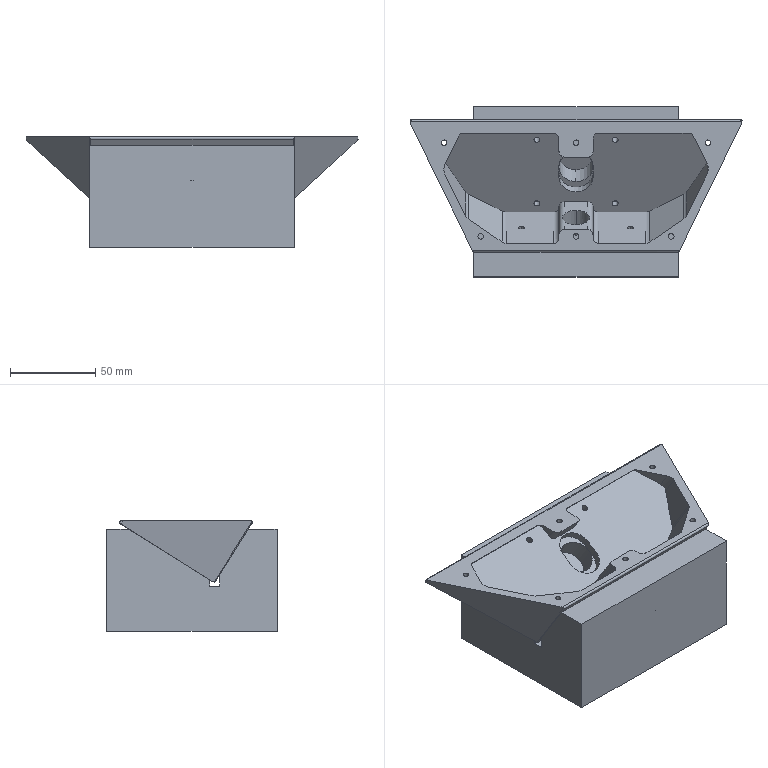NC program | Mastercam | posted with a generic post | part box 195.124 x 100 x 65 mm
Lines 1 to 1042 of 16336:
%
O0000()
(MATERIAL - ALUMINUM MM - 2024)
( T8 | 16 RC | H8 | D8 | WEAR COMP | TOOL DIA. - 16. | XY STOCK TO LEAVE - .15 | Z STOCK TO LEAVE - 0. )
( T2 | 16 FI | H2 | D2 | WEAR COMP | TOOL DIA. - 16. )
( T9 | 6 FEM | H9 | D9 | WEAR COMP | TOOL DIA. - 6. )
( T10 | 8 BM | H10 )
( T3 | 6 SPD | H3 )
( T11 | 10.3 DR | H11 )
( T12 | M12 X 1.75 RH | H12 )
( T13 | 10 FEMF | H13 | D13 | WEAR COMP | TOOL DIA. - 10. | XY STOCK TO LEAVE - .1 | Z STOCK TO LEAVE - 0. )
( T14 | 4.5 DR | H14 )
( T15 | 8 FEMR | H15 )
( T16 | 9 DR | H16 )
( T17 | 8 FEMF | H17 | D17 | WEAR COMP | TOOL DIA. - 8. | XY STOCK TO LEAVE - .05 | Z STOCK TO LEAVE - 0. )
( T18 | 14 FEM | H18 )
( T6 | 12 FEMR | H6 | XY STOCK TO LEAVE - .5 | Z STOCK TO LEAVE - .1 )
( T7 | 12 FEMF | H7 | XY STOCK TO LEAVE - .3 | Z STOCK TO LEAVE - 0. )
N100 G21
N110 G0 G17 G40 G49 G80 G90
N120 T8 M6
N130 G0 G90 G54 X82.95 Y-9.86 A0. S5500 M3
N140 G43 H8 Z50.
N150 Z1.
N160 G1 Z0. F2000.
N170 G41 D8 X68.95
N180 G3 X68.15 Y-10.66 I0. J-.8
N190 G1 Y-57.173 Z-.189
N200 G2 X60. Y-65.323 Z-.242 I-8.15 J0.
N210 G1 X-60. Z-.73
N220 G2 X-68.15 Y-57.173 Z-.782 I0. J8.15
N230 G1 Y42.828 Z-1.189
N240 G2 X-60. Y50.978 Z-1.242 I8.15 J0.
N250 G1 X60. Z-1.73
N260 G2 X68.15 Y42.828 Z-1.782 I0. J-8.15
N270 G1 Y-10.66 Z-2.
N280 Y-57.173 Z-2.189
N290 G2 X60. Y-65.323 Z-2.242 I-8.15 J0.
N300 G1 X-60. Z-2.73
N310 G2 X-68.15 Y-57.173 Z-2.782 I0. J8.15
N320 G1 Y42.828 Z-3.189
N330 G2 X-60. Y50.978 Z-3.242 I8.15 J0.
N340 G1 X60. Z-3.73
N350 G2 X68.15 Y42.828 Z-3.782 I0. J-8.15
N360 G1 Y-10.66 Z-4.
N370 Y-57.173 Z-4.189
N380 G2 X60. Y-65.323 Z-4.242 I-8.15 J0.
N390 G1 X-60. Z-4.73
N400 G2 X-68.15 Y-57.173 Z-4.782 I0. J8.15
N410 G1 Y42.828 Z-5.189
N420 G2 X-60. Y50.978 Z-5.242 I8.15 J0.
N430 G1 X60. Z-5.73
N440 G2 X68.15 Y42.828 Z-5.782 I0. J-8.15
N450 G1 Y-10.66 Z-6.
N460 Y-57.173 Z-6.189
N470 G2 X60. Y-65.323 Z-6.242 I-8.15 J0.
N480 G1 X-60. Z-6.73
N490 G2 X-68.15 Y-57.173 Z-6.782 I0. J8.15
N500 G1 Y42.828 Z-7.189
N510 G2 X-60. Y50.978 Z-7.242 I8.15 J0.
N520 G1 X60. Z-7.73
N530 G2 X68.15 Y42.828 Z-7.782 I0. J-8.15
N540 G1 Y-10.66 Z-8.
N550 Y-57.173 Z-8.189
N560 G2 X60. Y-65.323 Z-8.242 I-8.15 J0.
N570 G1 X-60. Z-8.73
N580 G2 X-68.15 Y-57.173 Z-8.782 I0. J8.15
N590 G1 Y42.828 Z-9.189
N600 G2 X-60. Y50.978 Z-9.242 I8.15 J0.
N610 G1 X60. Z-9.73
N620 G2 X68.15 Y42.828 Z-9.782 I0. J-8.15
N630 G1 Y-10.66 Z-10.
N640 Y-57.173 Z-10.189
N650 G2 X60. Y-65.323 Z-10.242 I-8.15 J0.
N660 G1 X-60. Z-10.73
N670 G2 X-68.15 Y-57.173 Z-10.782 I0. J8.15
N680 G1 Y42.828 Z-11.189
N690 G2 X-60. Y50.978 Z-11.242 I8.15 J0.
N700 G1 X60. Z-11.73
N710 G2 X68.15 Y42.828 Z-11.782 I0. J-8.15
N720 G1 Y-10.66 Z-12.
N730 Y-57.173 Z-12.189
N740 G2 X60. Y-65.323 Z-12.242 I-8.15 J0.
N750 G1 X-60. Z-12.73
N760 G2 X-68.15 Y-57.173 Z-12.782 I0. J8.15
N770 G1 Y42.828 Z-13.189
N780 G2 X-60. Y50.978 Z-13.242 I8.15 J0.
N790 G1 X60. Z-13.73
N800 G2 X68.15 Y42.828 Z-13.782 I0. J-8.15
N810 G1 Y-10.66 Z-14.
N820 Y-57.173 Z-14.189
N830 G2 X60. Y-65.323 Z-14.242 I-8.15 J0.
N840 G1 X-60. Z-14.73
N850 G2 X-68.15 Y-57.173 Z-14.782 I0. J8.15
N860 G1 Y42.828 Z-15.189
N870 G2 X-60. Y50.978 Z-15.242 I8.15 J0.
N880 G1 X60. Z-15.73
N890 G2 X68.15 Y42.828 Z-15.782 I0. J-8.15
N900 G1 Y-10.66 Z-16.
N910 Y-57.173 Z-16.189
N920 G2 X60. Y-65.323 Z-16.242 I-8.15 J0.
N930 G1 X-60. Z-16.73
N940 G2 X-68.15 Y-57.173 Z-16.782 I0. J8.15
N950 G1 Y42.828 Z-17.189
N960 G2 X-60. Y50.978 Z-17.242 I8.15 J0.
N970 G1 X60. Z-17.73
N980 G2 X68.15 Y42.828 Z-17.782 I0. J-8.15
N990 G1 Y-10.66 Z-18.
N1000 Y-57.173 Z-18.189
N1010 G2 X60. Y-65.323 Z-18.242 I-8.15 J0.
N1020 G1 X-60. Z-18.73
N1030 G2 X-68.15 Y-57.173 Z-18.782 I0. J8.15
N1040 G1 Y42.828 Z-19.189
N1050 G2 X-60. Y50.978 Z-19.242 I8.15 J0.
N1060 G1 X60. Z-19.73
N1070 G2 X68.15 Y42.828 Z-19.782 I0. J-8.15
N1080 G1 Y-10.66 Z-20.
N1090 Y-57.173 Z-20.189
N1100 G2 X60. Y-65.323 Z-20.242 I-8.15 J0.
N1110 G1 X-60. Z-20.73
N1120 G2 X-68.15 Y-57.173 Z-20.782 I0. J8.15
N1130 G1 Y42.828 Z-21.189
N1140 G2 X-60. Y50.978 Z-21.242 I8.15 J0.
N1150 G1 X60. Z-21.73
N1160 G2 X68.15 Y42.828 Z-21.782 I0. J-8.15
N1170 G1 Y-10.66 Z-22.
N1180 Y-57.173 Z-22.189
N1190 G2 X60. Y-65.323 Z-22.242 I-8.15 J0.
N1200 G1 X-60. Z-22.73
N1210 G2 X-68.15 Y-57.173 Z-22.782 I0. J8.15
N1220 G1 Y42.828 Z-23.189
N1230 G2 X-60. Y50.978 Z-23.242 I8.15 J0.
N1240 G1 X60. Z-23.73
N1250 G2 X68.15 Y42.828 Z-23.782 I0. J-8.15
N1260 G1 Y-10.66 Z-24.
N1270 Y-57.173 Z-24.189
N1280 G2 X60. Y-65.323 Z-24.242 I-8.15 J0.
N1290 G1 X-60. Z-24.73
N1300 G2 X-68.15 Y-57.173 Z-24.782 I0. J8.15
N1310 G1 Y42.828 Z-25.189
N1320 G2 X-60. Y50.978 Z-25.242 I8.15 J0.
N1330 G1 X60. Z-25.73
N1340 G2 X68.15 Y42.828 Z-25.782 I0. J-8.15
N1350 G1 Y-10.66 Z-26.
N1360 Y-57.173 Z-26.189
N1370 G2 X60. Y-65.323 Z-26.242 I-8.15 J0.
N1380 G1 X-60. Z-26.73
N1390 G2 X-68.15 Y-57.173 Z-26.782 I0. J8.15
N1400 G1 Y42.828 Z-27.189
N1410 G2 X-60. Y50.978 Z-27.242 I8.15 J0.
N1420 G1 X60. Z-27.73
N1430 G2 X68.15 Y42.828 Z-27.782 I0. J-8.15
N1440 G1 Y-10.66 Z-28.
N1450 Y-57.173 Z-28.189
N1460 G2 X60. Y-65.323 Z-28.242 I-8.15 J0.
N1470 G1 X-60. Z-28.73
N1480 G2 X-68.15 Y-57.173 Z-28.782 I0. J8.15
N1490 G1 Y42.828 Z-29.189
N1500 G2 X-60. Y50.978 Z-29.242 I8.15 J0.
N1510 G1 X60. Z-29.73
N1520 G2 X68.15 Y42.828 Z-29.782 I0. J-8.15
N1530 G1 Y-10.66 Z-30.
N1540 Y-57.173 Z-30.189
N1550 G2 X60. Y-65.323 Z-30.242 I-8.15 J0.
N1560 G1 X-60. Z-30.73
N1570 G2 X-68.15 Y-57.173 Z-30.782 I0. J8.15
N1580 G1 Y42.828 Z-31.189
N1590 G2 X-60. Y50.978 Z-31.242 I8.15 J0.
N1600 G1 X60. Z-31.73
N1610 G2 X68.15 Y42.828 Z-31.782 I0. J-8.15
N1620 G1 Y-10.66 Z-32.
N1630 Y-57.173 Z-32.189
N1640 G2 X60. Y-65.323 Z-32.242 I-8.15 J0.
N1650 G1 X-60. Z-32.73
N1660 G2 X-68.15 Y-57.173 Z-32.782 I0. J8.15
N1670 G1 Y42.828 Z-33.189
N1680 G2 X-60. Y50.978 Z-33.242 I8.15 J0.
N1690 G1 X60. Z-33.73
N1700 G2 X68.15 Y42.828 Z-33.782 I0. J-8.15
N1710 G1 Y-10.66 Z-34.
N1720 Y-57.173 Z-34.189
N1730 G2 X60. Y-65.323 Z-34.242 I-8.15 J0.
N1740 G1 X-60. Z-34.73
N1750 G2 X-68.15 Y-57.173 Z-34.782 I0. J8.15
N1760 G1 Y42.828 Z-35.189
N1770 G2 X-60. Y50.978 Z-35.242 I8.15 J0.
N1780 G1 X60. Z-35.73
N1790 G2 X68.15 Y42.828 Z-35.782 I0. J-8.15
N1800 G1 Y-10.66 Z-36.
N1810 Y-57.173 Z-36.189
N1820 G2 X60. Y-65.323 Z-36.242 I-8.15 J0.
N1830 G1 X-60. Z-36.73
N1840 G2 X-68.15 Y-57.173 Z-36.782 I0. J8.15
N1850 G1 Y42.828 Z-37.189
N1860 G2 X-60. Y50.978 Z-37.242 I8.15 J0.
N1870 G1 X60. Z-37.73
N1880 G2 X68.15 Y42.828 Z-37.782 I0. J-8.15
N1890 G1 Y-10.66 Z-38.
N1900 Y-57.173 Z-38.189
N1910 G2 X60. Y-65.323 Z-38.242 I-8.15 J0.
N1920 G1 X-60. Z-38.73
N1930 G2 X-68.15 Y-57.173 Z-38.782 I0. J8.15
N1940 G1 Y42.828 Z-39.189
N1950 G2 X-60. Y50.978 Z-39.242 I8.15 J0.
N1960 G1 X60. Z-39.73
N1970 G2 X68.15 Y42.828 Z-39.782 I0. J-8.15
N1980 G1 Y-10.66 Z-40.
N1990 Y-57.173 Z-40.189
N2000 G2 X60. Y-65.323 Z-40.242 I-8.15 J0.
N2010 G1 X-60. Z-40.73
N2020 G2 X-68.15 Y-57.173 Z-40.782 I0. J8.15
N2030 G1 Y42.828 Z-41.189
N2040 G2 X-60. Y50.978 Z-41.242 I8.15 J0.
N2050 G1 X60. Z-41.73
N2060 G2 X68.15 Y42.828 Z-41.782 I0. J-8.15
N2070 G1 Y-10.66 Z-42.
N2080 Y-57.173 Z-42.189
N2090 G2 X60. Y-65.323 Z-42.242 I-8.15 J0.
N2100 G1 X-60. Z-42.73
N2110 G2 X-68.15 Y-57.173 Z-42.782 I0. J8.15
N2120 G1 Y42.828 Z-43.189
N2130 G2 X-60. Y50.978 Z-43.242 I8.15 J0.
N2140 G1 X60. Z-43.73
N2150 G2 X68.15 Y42.828 Z-43.782 I0. J-8.15
N2160 G1 Y-10.66 Z-44.
N2170 Y-57.173 Z-44.189
N2180 G2 X60. Y-65.323 Z-44.242 I-8.15 J0.
N2190 G1 X-60. Z-44.73
N2200 G2 X-68.15 Y-57.173 Z-44.782 I0. J8.15
N2210 G1 Y42.828 Z-45.189
N2220 G2 X-60. Y50.978 Z-45.242 I8.15 J0.
N2230 G1 X60. Z-45.73
N2240 G2 X68.15 Y42.828 Z-45.782 I0. J-8.15
N2250 G1 Y-10.66 Z-46.
N2260 Y-57.173 Z-46.189
N2270 G2 X60. Y-65.323 Z-46.242 I-8.15 J0.
N2280 G1 X-60. Z-46.73
N2290 G2 X-68.15 Y-57.173 Z-46.782 I0. J8.15
N2300 G1 Y42.828 Z-47.189
N2310 G2 X-60. Y50.978 Z-47.242 I8.15 J0.
N2320 G1 X60. Z-47.73
N2330 G2 X68.15 Y42.828 Z-47.782 I0. J-8.15
N2340 G1 Y-10.66 Z-48.
N2350 Y-57.173 Z-48.189
N2360 G2 X60. Y-65.323 Z-48.242 I-8.15 J0.
N2370 G1 X-60. Z-48.73
N2380 G2 X-68.15 Y-57.173 Z-48.782 I0. J8.15
N2390 G1 Y42.828 Z-49.189
N2400 G2 X-60. Y50.978 Z-49.242 I8.15 J0.
N2410 G1 X60. Z-49.73
N2420 G2 X68.15 Y42.828 Z-49.782 I0. J-8.15
N2430 G1 Y-10.66 Z-50.
N2440 Y-57.173 Z-50.189
N2450 G2 X60. Y-65.323 Z-50.242 I-8.15 J0.
N2460 G1 X-60. Z-50.73
N2470 G2 X-68.15 Y-57.173 Z-50.782 I0. J8.15
N2480 G1 Y42.828 Z-51.189
N2490 G2 X-60. Y50.978 Z-51.242 I8.15 J0.
N2500 G1 X60. Z-51.73
N2510 G2 X68.15 Y42.828 Z-51.782 I0. J-8.15
N2520 G1 Y-10.66 Z-52.
N2530 Y-57.173 Z-52.189
N2540 G2 X60. Y-65.323 Z-52.242 I-8.15 J0.
N2550 G1 X-60. Z-52.73
N2560 G2 X-68.15 Y-57.173 Z-52.782 I0. J8.15
N2570 G1 Y42.828 Z-53.189
N2580 G2 X-60. Y50.978 Z-53.242 I8.15 J0.
N2590 G1 X60. Z-53.73
N2600 G2 X68.15 Y42.828 Z-53.782 I0. J-8.15
N2610 G1 Y-10.66 Z-54.
N2620 Y-57.173 Z-54.189
N2630 G2 X60. Y-65.323 Z-54.242 I-8.15 J0.
N2640 G1 X-60. Z-54.73
N2650 G2 X-68.15 Y-57.173 Z-54.782 I0. J8.15
N2660 G1 Y42.828 Z-55.189
N2670 G2 X-60. Y50.978 Z-55.242 I8.15 J0.
N2680 G1 X60. Z-55.73
N2690 G2 X68.15 Y42.828 Z-55.782 I0. J-8.15
N2700 G1 Y-10.66 Z-56.
N2710 Y-57.173 Z-56.189
N2720 G2 X60. Y-65.323 Z-56.242 I-8.15 J0.
N2730 G1 X-60. Z-56.73
N2740 G2 X-68.15 Y-57.173 Z-56.782 I0. J8.15
N2750 G1 Y42.828 Z-57.189
N2760 G2 X-60. Y50.978 Z-57.242 I8.15 J0.
N2770 G1 X60. Z-57.73
N2780 G2 X68.15 Y42.828 Z-57.782 I0. J-8.15
N2790 G1 Y-10.66 Z-58.
N2800 Y-57.173 Z-58.189
N2810 G2 X60. Y-65.323 Z-58.242 I-8.15 J0.
N2820 G1 X-60. Z-58.73
N2830 G2 X-68.15 Y-57.173 Z-58.782 I0. J8.15
N2840 G1 Y42.828 Z-59.189
N2850 G2 X-60. Y50.978 Z-59.242 I8.15 J0.
N2860 G1 X60. Z-59.73
N2870 G2 X68.15 Y42.828 Z-59.782 I0. J-8.15
N2880 G1 Y-10.66 Z-60.
N2890 Y-57.173 Z-60.189
N2900 G2 X60. Y-65.323 Z-60.242 I-8.15 J0.
N2910 G1 X-60. Z-60.73
N2920 G2 X-68.15 Y-57.173 Z-60.782 I0. J8.15
N2930 G1 Y-3.686 Z-61.
N2940 Y42.828
N2950 G2 X-60. Y50.978 I8.15 J0.
N2960 G1 X60.
N2970 G2 X68.15 Y42.828 I0. J-8.15
N2980 G1 Y-10.66
N2990 Y-57.173
N3000 G2 X60. Y-65.323 I-8.15 J0.
N3010 G1 X-60.
N3020 G2 X-68.15 Y-57.173 I0. J8.15
N3030 G1 Y-3.186
N3040 G3 X-68.95 Y-2.386 I-.8 J0.
N3050 G1 G40 X-82.95
N3060 G0 Z50.
N3070 X70. Y-5.183
N3080 Z5.3
N3090 G1 Z.3 F2000.
N3100 X62. Y-5.626
N3110 X-39.6 Y-11.242
N3120 X39.6
N3130 X38.8 Y-8.042
N3140 Y-2.442
N3150 X39.6 Y-.042
N3160 X-39.6
N3170 X-38.8 Y-3.242
N3180 Y-8.842
N3190 X-39.6 Y-11.242
N3200 X-51.6 Y-21.642
N3210 X51.6
N3220 X50.8 Y-18.442
N3230 Y8.758
N3240 X51.6 Y11.158
N3250 X-51.6
N3260 X-50.8 Y7.958
N3270 Y-19.242
N3280 X-51.6 Y-21.642
N3290 X-59.769 Y-31.797
N3300 X60.231
N3310 G2 X62. Y-32.04 I-.161 J-7.728
N3320 G1 Y21.614
N3330 G2 X60.209 Y21.367 I-1.985 J7.802
N3340 G1 X-59.793
N3350 G2 X-60.101 Y21.36 I-.308 J7.181
N3360 X-62. Y21.616 I0. J7.188
N3370 G1 Y-32.042
N3380 G2 X-60.003 Y-31.794 I1.997 J-7.913
N3390 X-59.769 Y-31.797 I0. J-8.161
N3400 G0 Z5.3
N3410 Z50.
N3420 X70. Y-5.183
N3430 Z4.307
N3440 G1 Z-.693 F2000.
N3450 X62. Y-5.58
N3460 X-39.6 Y-10.619
N3470 X39.6
N3480 X38.8 Y-7.419
N3490 Y-4.219
N3500 X39.6 Y-1.819
N3510 X-39.6
N3520 X-38.8 Y-5.019
N3530 Y-8.219
N3540 X-39.6 Y-10.619
N3550 X-51.6 Y-21.019
N3560 X51.6
N3570 X50.8 Y-17.819
N3580 Y6.981
N3590 X51.6 Y9.381
N3600 X-51.6
N3610 X-50.8 Y6.181
N3620 Y-18.619
N3630 X-51.6 Y-21.019
N3640 X-59.786 Y-31.175
N3650 X60.235
N3660 G2 X62. Y-31.418 I-.163 J-7.714
N3670 G1 Y20.024
N3680 G2 X60.207 Y19.778 I-1.985 J7.806
N3690 G1 X-59.793
N3700 G2 X-60.102 Y19.771 I-.309 J7.172
N3710 X-62. Y20.026 I0. J7.179
N3720 G1 Y-31.419
N3730 G2 X-60.013 Y-31.171 I1.987 J-7.845
N3740 X-59.786 Y-31.175 I0. J-8.093
N3750 G0 Z4.307
N3760 Z50.
N3770 X70. Y-5.183
N3780 Z3.313
N3790 G1 Z-1.687 F2000.
N3800 X62. Y-5.535
N3810 X-39.6 Y-9.999
N3820 X39.6
N3830 X38.8 Y-6.799
N3840 Y-5.199
N3850 X39.6 Y-2.799
N3860 X-39.6
N3870 X-38.8 Y-5.999
N3880 Y-7.599
N3890 X-39.6 Y-9.999
N3900 X-51.6 Y-20.399
N3910 X51.6
N3920 X50.8 Y-17.199
N3930 Y6.001
N3940 X51.6 Y8.401
N3950 X-51.6
N3960 X-50.8 Y5.201
N3970 Y-17.999
N3980 X-51.6 Y-20.399
N3990 X-59.806 Y-30.554
N4000 X60.235
N4010 G2 X62. Y-30.797 I-.163 J-7.715
N4020 G1 Y18.434
N4030 G2 X60.207 Y18.188 I-1.985 J7.806
N4040 G1 X-59.793
N4050 G2 X-60.102 Y18.181 I-.309 J7.172
N4060 X-62. Y18.437 I0. J7.179
N4070 G1 Y-30.799
N4080 G2 X-60.025 Y-30.552 I1.975 J-7.771
N4090 X-59.806 Y-30.554 I0. J-8.018
N4100 G0 Z3.313
N4110 Z50.
N4120 X70. Y-5.183
N4130 Z2.32
N4140 G1 Z-2.68 F2000.
N4150 X62. Y-5.489
N4160 X-39.6 Y-9.378
N4170 X39.6
N4180 Y-4.578
N4190 X-39.6
N4200 Y-9.378
N4210 X-51.6 Y-19.778
N4220 X51.6
N4230 X50.8 Y-16.578
N4240 Y4.222
N4250 X51.6 Y6.622
N4260 X-51.6
N4270 X-50.8 Y3.422
N4280 Y-17.378
N4290 X-51.6 Y-19.778
N4300 X-59.826 Y-29.934
N4310 X60.235 Y-29.933
N4320 G2 X62. Y-30.176 I-.163 J-7.715
N4330 G1 Y16.844
N4340 G2 X60.207 Y16.598 I-1.985 J7.807
N4350 G1 X-59.793
N4360 G2 X-60.102 Y16.591 I-.309 J7.173
N4370 X-62. Y16.847 I0. J7.18
N4380 G1 Y-30.178
N4390 G2 X-60.036 Y-29.931 I1.964 J-7.698
N4400 X-59.826 Y-29.934 I0. J-7.945
N4410 G0 Z2.32
N4420 Z50.
N4430 X70. Y-5.183
N4440 Z1.327
N4450 G1 Z-3.673 F2000.
N4460 X62. Y-5.444
N4470 X-39.6 Y-8.757
N4480 X39.6
N4490 Y-6.357
N4500 X-39.6
N4510 Y-8.757
N4520 X-51.6 Y-19.157
N4530 X51.6
N4540 X50.8 Y-15.957
N4550 Y2.443
N4560 X51.6 Y4.843
N4570 X-51.6
N4580 X-50.8 Y2.443
N4590 Y-16.757
N4600 X-51.6 Y-19.157
N4610 X-59.847 Y-29.314
N4620 X60.235 Y-29.313
N4630 G2 X62. Y-29.556 I-.163 J-7.714
N4640 G1 Y15.255
N4650 G2 X60.207 Y15.009 I-1.985 J7.806
N4660 G1 X-59.793
N4670 G2 X-60.102 Y15.002 I-.309 J7.172
N4680 X-62. Y15.257 I0. J7.179
N4690 G1 Y-29.557
N4700 G2 X-60.047 Y-29.311 I1.953 J-7.624
N4710 X-59.847 Y-29.314 I0. J-7.87
N4720 G0 Z1.327
N4730 Z50.
N4740 X70. Y-5.183
N4750 Z.333
N4760 G1 Z-4.667 F2000.
N4770 X62. Y-5.424
N4780 X-28.096 Y-8.137
N4790 X39.6
N4800 X-28.768
N4810 X-39.6
N4820 X-51.6 Y-18.537
N4830 X51.6
N4840 X50.8 Y-15.337
N4850 Y-.137
N4860 X51.6 Y3.063
N4870 X-51.6
N4880 X-50.8 Y.663
N4890 Y-16.137
N4900 X-51.6 Y-18.537
N4910 X-59.867 Y-28.693
N4920 X60.235 Y-28.692
N4930 G2 X62. Y-28.935 I-.163 J-7.715
N4940 G1 Y13.665
N4950 G2 X60.207 Y13.419 I-1.985 J7.806
N4960 G1 X-59.793
N4970 G2 X-60.102 Y13.412 I-.309 J7.172
N4980 X-62. Y13.668 I0. J7.179
N4990 G1 Y-28.937
N5000 G2 X-60.058 Y-28.691 I1.942 J-7.55
N5010 X-59.867 Y-28.693 I0. J-7.796
N5020 G0 Z.333
N5030 Z50.
N5040 X70. Y-5.183
N5050 Z-.66
N5060 G1 Z-5.66 F2000.
N5070 X62. Y-5.441
N5080 X-27.255 Y-8.316
N5090 X39.134
N5100 X-27.63
N5110 X-39.134
N5120 X-51.6 Y-17.916
N5130 X51.6
N5140 X50.8 Y-14.716
N5150 Y-1.116
N5160 X51.6 Y2.084
N5170 X-51.6
N5180 X-50.8 Y-.316
N5190 Y-15.516
N5200 X-51.6 Y-17.916
N5210 X-59.765 Y-28.071
N5220 X60.235
N5230 G2 X62. Y-28.314 I-.163 J-7.715
N5240 G1 Y12.075
N5250 G2 X60.207 Y11.829 I-1.985 J7.807
N5260 G1 X-59.793
N5270 G2 X-60.102 Y11.822 I-.309 J7.173
N5280 X-62. Y12.078 I0. J7.18
N5290 G1 Y-28.316
N5300 G2 X-60.003 Y-28.068 I1.997 J-7.918
N5310 X-59.765 Y-28.071 I0. J-8.166
N5320 G0 Z-.66
N5330 Z50.
N5340 X70. Y-5.183
N5350 Z-1.653
N5360 G1 Z-6.653 F2000.
N5370 X62. Y-5.486
N5380 X-38.8 Y-9.295
N5390 X38.8
N5400 Y-8.495
N5410 X-38.8
N5420 Y-9.295
N5430 X-51.6 Y-17.295
N5440 X51.6
N5450 X50.8 Y-14.095
N5460 Y-2.095
N5470 X51.6 Y.305
N5480 X-51.6
N5490 X-50.8 Y-2.895
N5500 Y-14.895
N5510 X-51.6 Y-17.295
N5520 X-59.765 Y-27.451
N5530 X60.235
N5540 G2 X62. Y-27.694 I-.163 J-7.714
N5550 G1 Y10.486
N5560 G2 X60.207 Y10.24 I-1.985 J7.806
N5570 G1 X-59.793
N5580 G2 X-60.102 Y10.233 I-.309 J7.172
N5590 X-62. Y10.488 I0. J7.179
N5600 G1 Y-27.695
N5610 G2 X-60.003 Y-27.447 I1.997 J-7.918
N5620 X-59.765 Y-27.451 I0. J-8.166
N5630 G0 Z-1.653
N5640 Z50.
N5650 X70. Y-5.183
N5660 Z-2.647
N5670 G1 Z-7.647 F2000.
N5680 X62. Y-5.939
N5690 X-51.6 Y-16.674
N5700 X51.6
N5710 X50.8 Y-13.474
N5720 Y-3.874
N5730 X51.6 Y-1.474
N5740 X-51.6
N5750 X-50.8 Y-4.674
N5760 Y-14.274
N5770 X-51.6 Y-16.674
N5780 X-59.765 Y-26.83
N5790 X60.235
N5800 G2 X62. Y-27.073 I-.163 J-7.714
N5810 G1 Y8.896
N5820 G2 X60.207 Y8.65 I-1.985 J7.806
N5830 G1 X-59.793
N5840 G2 X-60.102 Y8.643 I-.309 J7.172
N5850 X-62. Y8.899 I0. J7.179
N5860 G1 Y-27.074
N5870 G2 X-60.003 Y-26.826 I1.997 J-7.918
N5880 X-59.765 Y-26.83 I0. J-8.166
N5890 G0 Z-2.647
N5900 Z50.
N5910 X70. Y-5.183
N5920 Z-3.64
N5930 G1 Z-8.64 F2000.
N5940 X62. Y-5.898
N5950 X-51.6 Y-16.054
N5960 X51.6
N5970 X50.8 Y-12.854
N5980 Y-6.454
N5990 X51.6 Y-3.254
N6000 X-51.6
N6010 X-50.8 Y-5.654
N6020 Y-13.654
N6030 X-51.6 Y-16.054
N6040 X-59.765 Y-26.209
N6050 X60.235
N6060 G2 X62. Y-26.452 I-.163 J-7.715
N6070 G1 Y7.306
N6080 G2 X60.207 Y7.06 I-1.985 J7.807
N6090 G1 X-59.793
N6100 G2 X-60.102 Y7.053 I-.309 J7.173
N6110 X-62. Y7.309 I0. J7.18
N6120 G1 Y-26.454
N6130 G2 X-60.003 Y-26.206 I1.997 J-7.918
N6140 X-59.765 Y-26.209 I0. J-8.166
N6150 G0 Z-3.64
N6160 Z50.
N6170 X70. Y-5.183
N6180 Z-4.633
N6190 G1 Z-9.633 F2000.
N6200 X62. Y-5.858
N6210 X-51.6 Y-15.433
N6220 X51.6
N6230 X50.8 Y-12.233
N6240 Y-6.633
N6250 X51.6 Y-4.233
N6260 X-51.6
N6270 X-50.8 Y-7.433
N6280 Y-13.033
N6290 X-51.6 Y-15.433
N6300 X-59.765 Y-25.588
N6310 X60.235
N6320 G2 X62. Y-25.831 I-.163 J-7.715
N6330 G1 Y5.717
N6340 G2 X60.207 Y5.471 I-1.985 J7.806
N6350 G1 X-59.793
N6360 G2 X-60.102 Y5.464 I-.309 J7.172
N6370 X-62. Y5.719 I0. J7.179
N6380 G1 Y-25.833
N6390 G2 X-60.003 Y-25.585 I1.997 J-7.918
N6400 X-59.765 Y-25.588 I0. J-8.166
N6410 G0 Z-4.633
N6420 Z50.
N6430 X70. Y-5.183
N6440 Z-5.627
N6450 G1 Z-10.627 F2000.
N6460 X62. Y-5.817
N6470 X-51.6 Y-14.812
N6480 X51.6
N6490 X50.8 Y-11.612
N6500 Y-8.412
N6510 X51.6 Y-6.012
N6520 X-51.6
N6530 X-50.8 Y-9.212
N6540 Y-12.412
N6550 X-51.6 Y-14.812
N6560 X-59.765 Y-24.968
N6570 X60.235
N6580 G2 X62. Y-25.211 I-.163 J-7.714
N6590 G1 Y4.127
N6600 G2 X60.207 Y3.881 I-1.985 J7.806
N6610 G1 X-59.793
N6620 G2 X-60.102 Y3.874 I-.309 J7.172
N6630 X-62. Y4.13 I0. J7.179
N6640 G1 Y-25.212
N6650 G2 X-60.003 Y-24.964 I1.997 J-7.918
N6660 X-59.765 Y-24.968 I0. J-8.166
N6670 G0 Z-5.627
N6680 Z50.
N6690 X70. Y-5.183
N6700 Z-6.62
N6710 G1 Z-11.62 F2000.
N6720 X62. Y-5.776
N6730 X-51.6 Y-14.192
N6740 X51.6
N6750 X50.8 Y-11.792
N6760 Y-10.192
N6770 X51.6 Y-7.792
N6780 X-51.6
N6790 X-50.8 Y-10.992
N6800 X-51.6 Y-14.192
N6810 X-59.765 Y-24.347
N6820 X60.235
N6830 G2 X62. Y-24.59 I-.163 J-7.715
N6840 G1 Y2.537
N6850 G2 X60.207 Y2.291 I-1.985 J7.807
N6860 G1 X-59.793
N6870 G2 X-60.102 Y2.284 I-.309 J7.173
N6880 X-62. Y2.54 I0. J7.18
N6890 G1 Y-24.592
N6900 G2 X-60.003 Y-24.344 I1.997 J-7.917
N6910 X-59.765 Y-24.347 I0. J-8.165
N6920 G0 Z-6.62
N6930 Z50.
N6940 X70. Y-5.183
N6950 Z-7.613
N6960 G1 Z-12.613 F2000.
N6970 X62. Y-5.735
N6980 X-51.6 Y-13.571
N6990 X51.6
N7000 Y-9.571
N7010 X-51.6
N7020 Y-13.571
N7030 X-59.765 Y-23.726
N7040 X60.235
N7050 G2 X62. Y-23.969 I-.163 J-7.715
N7060 G1 Y.948
N7070 G2 X60.207 Y.702 I-1.985 J7.806
N7080 G1 X-59.793
N7090 G2 X-60.102 Y.695 I-.309 J7.172
N7100 X-62. Y.95 I0. J7.179
N7110 G1 Y-23.971
N7120 G2 X-60.003 Y-23.723 I1.997 J-7.918
N7130 X-59.765 Y-23.726 I0. J-8.166
N7140 G0 Z-7.613
N7150 Z50.
N7160 X70. Y-5.183
N7170 Z-8.607
N7180 G1 Z-13.607 F2000.
N7190 X62. Y-5.694
N7200 X-51.6 Y-12.95
N7210 X51.6
N7220 Y-10.55
N7230 X-51.6
N7240 Y-12.95
N7250 X-59.765 Y-23.106
N7260 X60.235
N7270 G2 X62. Y-23.349 I-.163 J-7.714
N7280 G1 Y-.642
N7290 G2 X60.207 Y-.888 I-1.985 J7.806
N7300 G1 X-59.793
N7310 G2 X-60.102 Y-.895 I-.309 J7.172
N7320 X-62. Y-.639 I0. J7.179
N7330 G1 Y-23.35
N7340 G2 X-60.003 Y-23.102 I1.997 J-7.918
N7350 X-59.765 Y-23.106 I0. J-8.166
N7360 G0 Z-8.607
N7370 Z50.
N7380 X70. Y-5.183
N7390 Z-9.6
N7400 G1 Z-14.6 F2000.
N7410 X62. Y-5.703
N7420 X-40.096 Y-12.33
N7430 X51.6
N7440 X-40.768
N7450 X-51.6
N7460 X-59.793 Y-2.478
N7470 G2 X-60.102 Y-2.485 I-.309 J7.173
N7480 X-62. Y-2.229 I0. J7.18
N7490 G1 Y-22.73
N7500 G2 X-60.003 Y-22.482 I1.997 J-7.917
N7510 X-59.765 Y-22.485 I0. J-8.165
N7520 G1 X60.235
N7530 G2 X62. Y-22.728 I-.163 J-7.715
N7540 G1 Y-2.232
N7550 G2 X60.207 Y-2.478 I-1.985 J7.807
N7560 G1 X-59.793
N7570 G0 Z-9.6
N7580 Z50.
N7590 X70. Y-5.183
N7600 Z-10.593
N7610 G1 Z-15.593 F2000.
N7620 X62. Y-5.721
N7630 X-50.881 Y-13.309
N7640 X50.881
N7650 Y-12.509
N7660 X-50.881
N7670 Y-13.309
N7680 X-59.765 Y-21.864
N7690 X60.235
N7700 G2 X62. Y-22.107 I-.163 J-7.715
N7710 G1 Y-3.821
N7720 G2 X60.207 Y-4.067 I-1.985 J7.806
N7730 G1 X-59.793
N7740 G2 X-60.102 Y-4.074 I-.309 J7.172
N7750 X-62. Y-3.819 I0. J7.179
N7760 G1 Y-22.109
N7770 G2 X-60.003 Y-21.861 I1.997 J-7.918
N7780 X-59.765 Y-21.864 I0. J-8.166
N7790 G0 Z-10.593
N7800 Z50.
N7810 X70. Y-5.183
N7820 Z-11.587
N7830 G1 Z-16.587 F2000.
N7840 X62. Y-9.336
N7850 X54. Y-13.488
N7860 X45.2
N7870 X33.2
N7880 X21.2
N7890 X9.2
N7900 X-2.8
N7910 X-14.8
N7920 X-26.8
N7930 X-38.8
N7940 X-50.8
N7950 X-59.765 Y-21.244
N7960 X60.235
N7970 G2 X62. Y-21.486 I-.163 J-7.714
N7980 G1 Y-5.411
N7990 G2 X60.207 Y-5.657 I-1.985 J7.806
N8000 G1 X-59.793
N8010 G2 X-60.102 Y-5.664 I-.309 J7.172
N8020 X-62. Y-5.408 I0. J7.179
N8030 G1 Y-21.488
N8040 G2 X-60.003 Y-21.24 I1.997 J-7.918
N8050 X-59.765 Y-21.244 I0. J-8.166
N8060 G0 Z-11.587
N8070 Z50.
N8080 X70. Y-5.183
N8090 Z-12.58
N8100 G1 Z-17.58 F2000.
N8110 X62. Y-7.001
N8120 G2 X60.207 Y-7.247 I-1.985 J7.807
N8130 G1 X-59.793
N8140 G2 X-60.102 Y-7.254 I-.309 J7.173
N8150 X-62. Y-6.998 I0. J7.18
N8160 G1 Y-20.867
N8170 G2 X-60.003 Y-20.619 I1.997 J-7.918
N8180 X-59.765 Y-20.623 I0. J-8.166
N8190 G1 X60.235
N8200 G2 X62. Y-20.866 I-.163 J-7.714
N8210 G1 Y-7.001
N8220 G0 Z-12.58
N8230 Z50.
N8240 X70. Y-5.183
N8250 Z-13.573
N8260 G1 Z-18.518 F2000.
N8270 X62. Y-8.59
N8280 Z-18.573
N8290 G2 X60.207 Y-8.836 I-1.985 J7.806
N8300 G1 X-59.793
N8310 G2 X-60.102 Y-8.843 I-.309 J7.172
N8320 X-62. Y-8.588 I0. J7.179
N8330 G1 Y-20.247
N8340 G2 X-60.003 Y-19.999 I1.997 J-7.918
N8350 X-59.765 Y-20.002 I0. J-8.166
N8360 G1 X60.235
N8370 G2 X62. Y-20.245 I-.163 J-7.715
N8380 G1 Y-8.59
N8390 G0 Z-13.573
N8400 Z50.
N8410 X70. Y-5.183
N8420 Z-14.567
N8430 G1 Z-19.278 F2000.
N8440 X62. Y-10.18
N8450 Z-19.567
N8460 G2 X60.207 Y-10.426 I-1.985 J7.806
N8470 G1 X-59.793
N8480 G2 X-60.102 Y-10.433 I-.309 J7.172
N8490 X-62. Y-10.177 I0. J7.179
N8500 G1 Y-19.626
N8510 G2 X-60.003 Y-19.378 I1.997 J-7.918
N8520 X-59.765 Y-19.381 I0. J-8.166
N8530 G1 X60.235
N8540 G2 X62. Y-19.624 I-.163 J-7.715
N8550 G1 Y-10.18
N8560 G0 Z-14.567
N8570 Z50.
N8580 X70. Y-5.183
N8590 Z-15.56
N8600 G1 Z-19.919 F2000.
N8610 X62. Y-11.77
N8620 Z-20.56
N8630 G2 X60.207 Y-12.016 I-1.985 J7.807
N8640 G1 X-59.793
N8650 G2 X-60.102 Y-12.023 I-.309 J7.173
N8660 X-62. Y-11.767 I0. J7.18
N8670 G1 Y-19.005
N8680 G2 X-60.003 Y-18.757 I1.997 J-7.918
N8690 X-59.765 Y-18.761 I0. J-8.166
N8700 G1 X60.235
N8710 G2 X62. Y-19.004 I-.163 J-7.714
N8720 G1 Y-11.77
N8730 G0 Z-15.56
N8740 Z50.
N8750 X70. Y-5.183
N8760 Z-16.553
N8770 G1 Z-20.464 F2000.
N8780 X62. Y-13.359
N8790 Z-21.553
N8800 G2 X60.207 Y-13.605 I-1.985 J7.806
N8810 G1 X-59.793
N8820 G2 X-60.102 Y-13.612 I-.309 J7.172
N8830 X-62. Y-13.357 I0. J7.179
N8840 G1 Y-18.385
N8850 G2 X-60.003 Y-18.137 I1.997 J-7.917
N8860 X-59.765 Y-18.14 I0. J-8.165
N8870 G1 X60.235
N8880 G2 X62. Y-18.383 I-.163 J-7.715
N8890 G1 Y-13.359
N8900 G0 Z-16.553
N8910 Z50.
N8920 X70. Y-5.183
N8930 Z-17.547
N8940 G1 Z-20.943 F2000.
N8950 X62. Y-14.949
N8960 Z-22.547
N8970 G2 X60.207 Y-15.195 I-1.985 J7.806
N8980 G1 X-59.793
N8990 G2 X-60.102 Y-15.202 I-.309 J7.172
N9000 X-62. Y-14.946 I0. J7.179
N9010 G1 Y-17.764
N9020 G2 X-60.003 Y-17.516 I1.997 J-7.918
N9030 X-59.765 Y-17.519 I0. J-8.166
N9040 G1 X60.235
N9050 G2 X62. Y-17.762 I-.163 J-7.715
N9060 G1 Y-14.949
N9070 G0 Z-17.547
N9080 Z50.
N9090 X70. Y-5.183
N9100 Z-18.54
N9110 G1 Z-21.346 F2000.
N9120 X62. Y-16.539
N9130 Z-23.54
N9140 G2 X60.207 Y-16.785 I-1.985 J7.807
N9150 G1 X-59.793
N9160 G2 X-60.102 Y-16.792 I-.309 J7.173
N9170 X-62. Y-16.536 I0. J7.18
N9180 G1 Y-17.143
N9190 G2 X-60.003 Y-16.895 I1.997 J-7.918
N9200 X-59.765 Y-16.899 I0. J-8.166
N9210 G1 X60.235
N9220 G2 X62. Y-17.142 I-.163 J-7.714
N9230 G1 Y-16.539
N9240 G0 Z-18.54
N9250 Z50.
N9260 M5
N9270 G91 G28 Z0.
N9280 A0.
N9290 M01
N9300 T2 M6
N9310 G0 G90 G17 G54 X82.8 Y-9.86 A0. S4000 M3
N9320 G43 H2 Z50.
N9330 Z-49.
N9340 G1 Z-61. F2000.
N9350 G41 D2 X68.8 F800.
N9360 G3 X68. Y-10.66 I0. J-.8
N9370 G1 Y-57.173
N9380 G2 X60. Y-65.173 I-8. J0.
N9390 G1 X-60.
N9400 G2 X-68. Y-57.173 I0. J8.
N9410 G1 Y42.828
N9420 G2 X-60. Y50.828 I8. J0.
N9430 G1 X60.
N9440 G2 X68. Y42.828 I0. J-8.
N9450 G1 Y-10.66
N9460 Y-11.16
N9470 G3 X68.8 Y-11.96 I.8 J0.
N9480 G1 G40 X82.8
N9490 Y-9.86
N9500 G41 D2 X68.8
N9510 G3 X68. Y-10.66 I0. J-.8
N9520 G1 Y-57.173
N9530 G2 X60. Y-65.173 I-8. J0.
N9540 G1 X-60.
N9550 G2 X-68. Y-57.173 I0. J8.
N9560 G1 Y42.828
N9570 G2 X-60. Y50.828 I8. J0.
N9580 G1 X60.
N9590 G2 X68. Y42.828 I0. J-8.
N9600 G1 Y-10.66
N9610 Y-11.16
N9620 G3 X68.8 Y-11.96 I.8 J0.
N9630 G1 G40 X82.8
N9640 G0 Z50.
N9650 M5
N9660 G91 G28 Z0.
N9670 A0.
N9680 M01
N9690 T9 M6
N9700 G0 G90 G17 G54 X-65.25 Y-20.53 A0. S5000 M3
N9710 G43 H9 Z50.
N9720 Z-21.966
N9730 G1 Z-23.716 F2000.
N9740 G41 D9 X-60. F1500.
N9750 X60.
N9760 G40 X65.25
N9770 Z-24.466 F2000.
N9780 G42 D9 X60. F1500.
N9790 X-60.
N9800 G40 X-65.25
N9810 Z-25.216 F2000.
N9820 G41 D9 X-60. F1500.
N9830 X60.
N9840 G40 X65.25
N9850 Z-25.966 F2000.
N9860 G42 D9 X60. F1500.
N9870 X-60.
N9880 G40 X-65.25
N9890 Z-26.716 F2000.
N9900 G41 D9 X-60. F1500.
N9910 X60.
N9920 G40 X65.25
N9930 Z-27.466 F2000.
N9940 G42 D9 X60. F1500.
N9950 X-60.
N9960 G40 X-65.25
N9970 Z-28.216 F2000.
N9980 G41 D9 X-60. F1500.
N9990 X60.
N100 G40 X65.25
N110 Z-28.966 F2000.
N120 G42 D9 X60. F1500.
N130 X-60.
N140 G40 X-65.25
N150 Z-29.716 F2000.
N160 G41 D9 X-60. F1500.
N170 X60.
N180 G40 X65.25
N190 Z-30.466 F2000.
N200 G42 D9 X60. F1500.
N210 X-60.
N220 G40 X-65.25
N230 Z-31.216 F2000.
N240 G41 D9 X-60. F1500.
N250 X60.
N260 G40 X65.25
N270 Z-31.966 F2000.
N280 G42 D9 X60. F1500.
N290 X-60.
N300 G40 X-65.25
N310 Z-32.716 F2000.
N320 G41 D9 X-60. F1500.
N330 X60.
N340 G40 X65.25
N350 Z-33.466 F2000.
N360 G42 D9 X60. F1500.
N370 X-60.
N380 G40 X-65.25
N390 G0 Z50.
N400 M5
N410 G91 G28 Z0.
N420 A0.
N430 M01